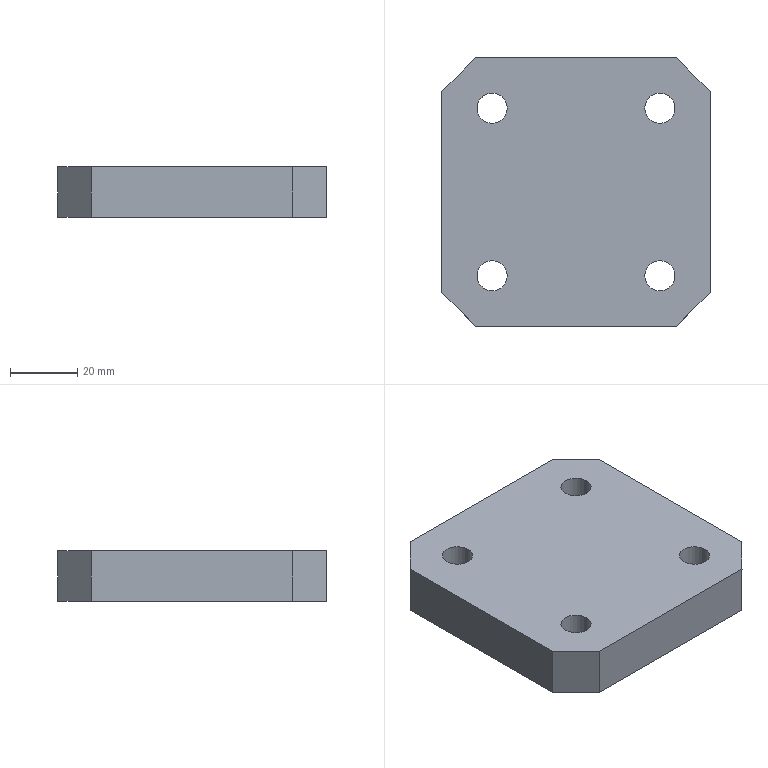Part | NX | features solid 2 | 1 solid | 14 faces | box 80 x 80 x 15 mm | volume 89183 mm3 | plane 10 | cylinder 4 | commonest cylinder face diameters 9 x4
STEP:
#1=CARTESIAN_POINT('',(-359.,-280.,315.));
#2=VERTEX_POINT('',#1);
#3=CARTESIAN_POINT('',(-419.,-280.,315.));
#4=VERTEX_POINT('',#3);
#5=CARTESIAN_POINT('',(9999577.414,-280.,315.));
#6=DIRECTION('',(-1.,0.,0.));
#7=VECTOR('',#6,1000.);
#8=LINE('',#5,#7);
#9=EDGE_CURVE('',#2,#4,#8,.T.);
#10=ORIENTED_EDGE('',*,*,#9,.T.);
#11=CARTESIAN_POINT('',(-419.,-280.,300.));
#12=VERTEX_POINT('',#11);
#13=CARTESIAN_POINT('',(-419.,-280.,300.));
#14=DIRECTION('',(0.,0.,-1.));
#15=VECTOR('',#14,1000.);
#16=LINE('',#13,#15);
#17=EDGE_CURVE('',#4,#12,#16,.T.);
#18=ORIENTED_EDGE('',*,*,#17,.T.);
#19=CARTESIAN_POINT('',(-359.,-280.,300.));
#20=VERTEX_POINT('',#19);
#21=CARTESIAN_POINT('',(9999577.414,-280.,300.));
#22=DIRECTION('',(-1.,0.,0.));
#23=VECTOR('',#22,1000.);
#24=LINE('',#21,#23);
#25=EDGE_CURVE('',#20,#12,#24,.T.);
#26=ORIENTED_EDGE('',*,*,#25,.F.);
#27=CARTESIAN_POINT('',(-359.,-280.,315.));
#28=DIRECTION('',(0.,0.,1.));
#29=VECTOR('',#28,1000.);
#30=LINE('',#27,#29);
#31=EDGE_CURVE('',#20,#2,#30,.T.);
#32=ORIENTED_EDGE('',*,*,#31,.T.);
#33=EDGE_LOOP('',(#10,#18,#26,#32));
#34=FACE_BOUND('',#33,.T.);
#35=CARTESIAN_POINT('',(9999577.414,-280.,315.));
#36=DIRECTION('',(0.,-1.,0.));
#37=DIRECTION('',(0.,0.,-1.));
#38=AXIS2_PLACEMENT_3D('',#35,#36,#37);
#39=PLANE('',#38);
#40=ADVANCED_FACE('',(#34),#39,.T.);
#41=CARTESIAN_POINT('',(-429.,-210.,300.));
#42=VERTEX_POINT('',#41);
#43=CARTESIAN_POINT('',(-429.,-270.,300.));
#44=VERTEX_POINT('',#43);
#45=CARTESIAN_POINT('',(-429.,-205.,300.));
#46=DIRECTION('',(0.,-1.,0.));
#47=VECTOR('',#46,1000.);
#48=LINE('',#45,#47);
#49=EDGE_CURVE('',#42,#44,#48,.T.);
#50=ORIENTED_EDGE('',*,*,#49,.T.);
#51=CARTESIAN_POINT('',(-429.,-270.,315.));
#52=VERTEX_POINT('',#51);
#53=CARTESIAN_POINT('',(-429.,-270.,315.));
#54=DIRECTION('',(0.,0.,1.));
#55=VECTOR('',#54,1000.);
#56=LINE('',#53,#55);
#57=EDGE_CURVE('',#44,#52,#56,.T.);
#58=ORIENTED_EDGE('',*,*,#57,.T.);
#59=CARTESIAN_POINT('',(-429.,-210.,315.));
#60=VERTEX_POINT('',#59);
#61=CARTESIAN_POINT('',(-429.,-205.,315.));
#62=DIRECTION('',(0.,-1.,0.));
#63=VECTOR('',#62,1000.);
#64=LINE('',#61,#63);
#65=EDGE_CURVE('',#60,#52,#64,.T.);
#66=ORIENTED_EDGE('',*,*,#65,.F.);
#67=CARTESIAN_POINT('',(-429.,-210.,315.));
#68=DIRECTION('',(0.,0.,-1.));
#69=VECTOR('',#68,1000.);
#70=LINE('',#67,#69);
#71=EDGE_CURVE('',#60,#42,#70,.T.);
#72=ORIENTED_EDGE('',*,*,#71,.T.);
#73=EDGE_LOOP('',(#50,#58,#66,#72));
#74=FACE_BOUND('',#73,.T.);
#75=CARTESIAN_POINT('',(-429.,-205.,315.));
#76=DIRECTION('',(1.,0.,0.));
#77=DIRECTION('',(0.,0.,-1.));
#78=AXIS2_PLACEMENT_3D('',#75,#76,#77);
#79=PLANE('',#78);
#80=ADVANCED_FACE('',(#74),#79,.F.);
#81=CARTESIAN_POINT('',(-359.,-200.,315.));
#82=VERTEX_POINT('',#81);
#83=CARTESIAN_POINT('',(-419.,-200.,315.));
#84=VERTEX_POINT('',#83);
#85=CARTESIAN_POINT('',(-359.,-200.,315.));
#86=CARTESIAN_POINT('',(-379.,-200.,315.));
#87=CARTESIAN_POINT('',(-399.,-200.,315.));
#88=CARTESIAN_POINT('',(-419.,-200.,315.));
#89=B_SPLINE_CURVE_WITH_KNOTS('',3,(#85,#86,#87,#88),.UNSPECIFIED.,.F.,.F.,(4,4),(0.125,0.875),.UNSPECIFIED.);
#90=EDGE_CURVE('',#82,#84,#89,.T.);
#91=ORIENTED_EDGE('',*,*,#90,.F.);
#92=CARTESIAN_POINT('',(-359.,-200.,300.));
#93=VERTEX_POINT('',#92);
#94=CARTESIAN_POINT('',(-359.,-200.,300.));
#95=DIRECTION('',(0.,0.,-1.));
#96=VECTOR('',#95,1000.);
#97=LINE('',#94,#96);
#98=EDGE_CURVE('',#82,#93,#97,.T.);
#99=ORIENTED_EDGE('',*,*,#98,.T.);
#100=CARTESIAN_POINT('',(-419.,-200.,300.));
#101=VERTEX_POINT('',#100);
#102=CARTESIAN_POINT('',(-419.,-200.,300.));
#103=CARTESIAN_POINT('',(-399.,-200.,300.));
#104=CARTESIAN_POINT('',(-379.,-200.,300.));
#105=CARTESIAN_POINT('',(-359.,-200.,300.));
#106=B_SPLINE_CURVE_WITH_KNOTS('',3,(#102,#103,#104,#105),.UNSPECIFIED.,.F.,.F.,(4,4),(0.125,0.875),.UNSPECIFIED.);
#107=EDGE_CURVE('',#93,#101,#106,.F.);
#108=ORIENTED_EDGE('',*,*,#107,.T.);
#109=CARTESIAN_POINT('',(-419.,-200.,315.));
#110=DIRECTION('',(0.,0.,1.));
#111=VECTOR('',#110,1000.);
#112=LINE('',#109,#111);
#113=EDGE_CURVE('',#101,#84,#112,.T.);
#114=ORIENTED_EDGE('',*,*,#113,.T.);
#115=EDGE_LOOP('',(#91,#99,#108,#114));
#116=FACE_BOUND('',#115,.T.);
#117=CARTESIAN_POINT('',(-355.414,-200.,315.));
#118=DIRECTION('',(0.,-1.,0.));
#119=DIRECTION('',(0.,0.,-1.));
#120=AXIS2_PLACEMENT_3D('',#117,#118,#119);
#121=PLANE('',#120);
#122=ADVANCED_FACE('',(#116),#121,.F.);
#123=CARTESIAN_POINT('',(-349.,-210.,315.));
#124=VERTEX_POINT('',#123);
#125=CARTESIAN_POINT('',(-349.,-270.,315.));
#126=VERTEX_POINT('',#125);
#127=CARTESIAN_POINT('',(-349.,9999726.414,315.));
#128=DIRECTION('',(0.,-1.,0.));
#129=VECTOR('',#128,1000.);
#130=LINE('',#127,#129);
#131=EDGE_CURVE('',#124,#126,#130,.T.);
#132=ORIENTED_EDGE('',*,*,#131,.T.);
#133=CARTESIAN_POINT('',(-349.,-270.,300.));
#134=VERTEX_POINT('',#133);
#135=CARTESIAN_POINT('',(-349.,-270.,315.));
#136=DIRECTION('',(0.,0.,-1.));
#137=VECTOR('',#136,1000.);
#138=LINE('',#135,#137);
#139=EDGE_CURVE('',#126,#134,#138,.T.);
#140=ORIENTED_EDGE('',*,*,#139,.T.);
#141=CARTESIAN_POINT('',(-349.,-210.,300.));
#142=VERTEX_POINT('',#141);
#143=CARTESIAN_POINT('',(-349.,9999726.414,300.));
#144=DIRECTION('',(0.,-1.,0.));
#145=VECTOR('',#144,1000.);
#146=LINE('',#143,#145);
#147=EDGE_CURVE('',#142,#134,#146,.T.);
#148=ORIENTED_EDGE('',*,*,#147,.F.);
#149=CARTESIAN_POINT('',(-349.,-210.,315.));
#150=DIRECTION('',(0.,0.,1.));
#151=VECTOR('',#150,1000.);
#152=LINE('',#149,#151);
#153=EDGE_CURVE('',#142,#124,#152,.T.);
#154=ORIENTED_EDGE('',*,*,#153,.T.);
#155=EDGE_LOOP('',(#132,#140,#148,#154));
#156=FACE_BOUND('',#155,.T.);
#157=CARTESIAN_POINT('',(-349.,9999726.414,315.));
#158=DIRECTION('',(1.,0.,0.));
#159=DIRECTION('',(0.,0.,-1.));
#160=AXIS2_PLACEMENT_3D('',#157,#158,#159);
#161=PLANE('',#160);
#162=ADVANCED_FACE('',(#156),#161,.T.);
#163=CARTESIAN_POINT('',(-359.504,-215.004,315.));
#164=VERTEX_POINT('',#163);
#165=CARTESIAN_POINT('',(-364.004,-215.004,315.));
#166=DIRECTION('',(0.,0.,1.));
#167=DIRECTION('',(1.,0.,0.));
#168=AXIS2_PLACEMENT_3D('',#165,#166,#167);
#169=CIRCLE('',#168,4.5);
#170=EDGE_CURVE('',#164,#164,#169,.T.);
#171=ORIENTED_EDGE('',*,*,#170,.F.);
#172=EDGE_LOOP('',(#171));
#173=FACE_BOUND('',#172,.T.);
#174=CARTESIAN_POINT('',(-409.496,-215.004,315.));
#175=VERTEX_POINT('',#174);
#176=CARTESIAN_POINT('',(-413.996,-215.004,315.));
#177=DIRECTION('',(0.,0.,1.));
#178=DIRECTION('',(1.,0.,0.));
#179=AXIS2_PLACEMENT_3D('',#176,#177,#178);
#180=CIRCLE('',#179,4.5);
#181=EDGE_CURVE('',#175,#175,#180,.T.);
#182=ORIENTED_EDGE('',*,*,#181,.F.);
#183=EDGE_LOOP('',(#182));
#184=FACE_BOUND('',#183,.T.);
#185=CARTESIAN_POINT('',(-409.496,-264.996,315.));
#186=VERTEX_POINT('',#185);
#187=CARTESIAN_POINT('',(-413.996,-264.996,315.));
#188=DIRECTION('',(0.,0.,1.));
#189=DIRECTION('',(1.,0.,0.));
#190=AXIS2_PLACEMENT_3D('',#187,#188,#189);
#191=CIRCLE('',#190,4.5);
#192=EDGE_CURVE('',#186,#186,#191,.T.);
#193=ORIENTED_EDGE('',*,*,#192,.F.);
#194=EDGE_LOOP('',(#193));
#195=FACE_BOUND('',#194,.T.);
#196=CARTESIAN_POINT('',(-359.504,-264.996,315.));
#197=VERTEX_POINT('',#196);
#198=CARTESIAN_POINT('',(-364.004,-264.996,315.));
#199=DIRECTION('',(0.,0.,1.));
#200=DIRECTION('',(1.,0.,0.));
#201=AXIS2_PLACEMENT_3D('',#198,#199,#200);
#202=CIRCLE('',#201,4.5);
#203=EDGE_CURVE('',#197,#197,#202,.T.);
#204=ORIENTED_EDGE('',*,*,#203,.F.);
#205=EDGE_LOOP('',(#204));
#206=FACE_BOUND('',#205,.T.);
#207=ORIENTED_EDGE('',*,*,#65,.T.);
#208=CARTESIAN_POINT('',(-424.707,-274.293,315.));
#209=DIRECTION('',(0.7071,-0.7071,0.));
#210=VECTOR('',#209,1000.);
#211=LINE('',#208,#210);
#212=EDGE_CURVE('',#52,#4,#211,.T.);
#213=ORIENTED_EDGE('',*,*,#212,.T.);
#214=ORIENTED_EDGE('',*,*,#9,.F.);
#215=CARTESIAN_POINT('',(-319.707,-240.707,315.));
#216=DIRECTION('',(-0.7071,-0.7071,0.));
#217=VECTOR('',#216,1000.);
#218=LINE('',#215,#217);
#219=EDGE_CURVE('',#2,#126,#218,.F.);
#220=ORIENTED_EDGE('',*,*,#219,.T.);
#221=ORIENTED_EDGE('',*,*,#131,.F.);
#222=CARTESIAN_POINT('',(-354.707,-204.293,315.));
#223=DIRECTION('',(-0.7071,0.7071,0.));
#224=VECTOR('',#223,1000.);
#225=LINE('',#222,#224);
#226=EDGE_CURVE('',#124,#82,#225,.T.);
#227=ORIENTED_EDGE('',*,*,#226,.T.);
#228=ORIENTED_EDGE('',*,*,#90,.T.);
#229=CARTESIAN_POINT('',(-389.707,-170.707,315.));
#230=DIRECTION('',(0.7071,0.7071,0.));
#231=VECTOR('',#230,1000.);
#232=LINE('',#229,#231);
#233=EDGE_CURVE('',#84,#60,#232,.F.);
#234=ORIENTED_EDGE('',*,*,#233,.T.);
#235=EDGE_LOOP('',(#207,#213,#214,#220,#221,#227,#228,#234));
#236=FACE_BOUND('',#235,.T.);
#237=CARTESIAN_POINT('',(-355.414,-205.,315.));
#238=DIRECTION('',(0.,0.,1.));
#239=DIRECTION('',(-1.,0.,0.));
#240=AXIS2_PLACEMENT_3D('',#237,#238,#239);
#241=PLANE('',#240);
#242=ADVANCED_FACE('',(#173,#184,#195,#206,#236),#241,.T.);
#243=CARTESIAN_POINT('',(-359.504,-215.004,300.));
#244=VERTEX_POINT('',#243);
#245=CARTESIAN_POINT('',(-364.004,-215.004,300.));
#246=DIRECTION('',(0.,0.,1.));
#247=DIRECTION('',(1.,0.,0.));
#248=AXIS2_PLACEMENT_3D('',#245,#246,#247);
#249=CIRCLE('',#248,4.5);
#250=EDGE_CURVE('',#244,#244,#249,.T.);
#251=ORIENTED_EDGE('',*,*,#250,.T.);
#252=EDGE_LOOP('',(#251));
#253=FACE_BOUND('',#252,.T.);
#254=CARTESIAN_POINT('',(-409.496,-215.004,300.));
#255=VERTEX_POINT('',#254);
#256=CARTESIAN_POINT('',(-413.996,-215.004,300.));
#257=DIRECTION('',(0.,0.,1.));
#258=DIRECTION('',(1.,0.,0.));
#259=AXIS2_PLACEMENT_3D('',#256,#257,#258);
#260=CIRCLE('',#259,4.5);
#261=EDGE_CURVE('',#255,#255,#260,.T.);
#262=ORIENTED_EDGE('',*,*,#261,.T.);
#263=EDGE_LOOP('',(#262));
#264=FACE_BOUND('',#263,.T.);
#265=CARTESIAN_POINT('',(-409.496,-264.996,300.));
#266=VERTEX_POINT('',#265);
#267=CARTESIAN_POINT('',(-413.996,-264.996,300.));
#268=DIRECTION('',(0.,0.,1.));
#269=DIRECTION('',(1.,0.,0.));
#270=AXIS2_PLACEMENT_3D('',#267,#268,#269);
#271=CIRCLE('',#270,4.5);
#272=EDGE_CURVE('',#266,#266,#271,.T.);
#273=ORIENTED_EDGE('',*,*,#272,.T.);
#274=EDGE_LOOP('',(#273));
#275=FACE_BOUND('',#274,.T.);
#276=CARTESIAN_POINT('',(-359.504,-264.996,300.));
#277=VERTEX_POINT('',#276);
#278=CARTESIAN_POINT('',(-364.004,-264.996,300.));
#279=DIRECTION('',(0.,0.,1.));
#280=DIRECTION('',(1.,0.,0.));
#281=AXIS2_PLACEMENT_3D('',#278,#279,#280);
#282=CIRCLE('',#281,4.5);
#283=EDGE_CURVE('',#277,#277,#282,.T.);
#284=ORIENTED_EDGE('',*,*,#283,.T.);
#285=EDGE_LOOP('',(#284));
#286=FACE_BOUND('',#285,.T.);
#287=ORIENTED_EDGE('',*,*,#25,.T.);
#288=CARTESIAN_POINT('',(-419.,-280.,300.));
#289=DIRECTION('',(-0.7071,0.7071,0.));
#290=VECTOR('',#289,1000.);
#291=LINE('',#288,#290);
#292=EDGE_CURVE('',#12,#44,#291,.T.);
#293=ORIENTED_EDGE('',*,*,#292,.T.);
#294=ORIENTED_EDGE('',*,*,#49,.F.);
#295=CARTESIAN_POINT('',(-429.,-210.,300.));
#296=DIRECTION('',(-0.7071,-0.7071,0.));
#297=VECTOR('',#296,1000.);
#298=LINE('',#295,#297);
#299=EDGE_CURVE('',#42,#101,#298,.F.);
#300=ORIENTED_EDGE('',*,*,#299,.T.);
#301=ORIENTED_EDGE('',*,*,#107,.F.);
#302=CARTESIAN_POINT('',(-359.,-200.,300.));
#303=DIRECTION('',(0.7071,-0.7071,0.));
#304=VECTOR('',#303,1000.);
#305=LINE('',#302,#304);
#306=EDGE_CURVE('',#93,#142,#305,.T.);
#307=ORIENTED_EDGE('',*,*,#306,.T.);
#308=ORIENTED_EDGE('',*,*,#147,.T.);
#309=CARTESIAN_POINT('',(-349.,-270.,300.));
#310=DIRECTION('',(0.7071,0.7071,0.));
#311=VECTOR('',#310,1000.);
#312=LINE('',#309,#311);
#313=EDGE_CURVE('',#134,#20,#312,.F.);
#314=ORIENTED_EDGE('',*,*,#313,.T.);
#315=EDGE_LOOP('',(#287,#293,#294,#300,#301,#307,#308,#314));
#316=FACE_BOUND('',#315,.T.);
#317=CARTESIAN_POINT('',(-355.414,-205.,300.));
#318=DIRECTION('',(0.,0.,1.));
#319=DIRECTION('',(-1.,0.,0.));
#320=AXIS2_PLACEMENT_3D('',#317,#318,#319);
#321=PLANE('',#320);
#322=ADVANCED_FACE('',(#253,#264,#275,#286,#316),#321,.F.);
#323=ORIENTED_EDGE('',*,*,#212,.F.);
#324=ORIENTED_EDGE('',*,*,#57,.F.);
#325=ORIENTED_EDGE('',*,*,#292,.F.);
#326=ORIENTED_EDGE('',*,*,#17,.F.);
#327=EDGE_LOOP('',(#323,#324,#325,#326));
#328=FACE_BOUND('',#327,.T.);
#329=CARTESIAN_POINT('',(-419.,-280.,315.));
#330=DIRECTION('',(-0.7071,-0.7071,0.));
#331=DIRECTION('',(0.7071,-0.7071,0.));
#332=AXIS2_PLACEMENT_3D('',#329,#330,#331);
#333=PLANE('',#332);
#334=ADVANCED_FACE('',(#328),#333,.T.);
#335=ORIENTED_EDGE('',*,*,#219,.F.);
#336=ORIENTED_EDGE('',*,*,#31,.F.);
#337=ORIENTED_EDGE('',*,*,#313,.F.);
#338=ORIENTED_EDGE('',*,*,#139,.F.);
#339=EDGE_LOOP('',(#335,#336,#337,#338));
#340=FACE_BOUND('',#339,.T.);
#341=CARTESIAN_POINT('',(-349.,-270.,315.));
#342=DIRECTION('',(-0.7071,0.7071,0.));
#343=DIRECTION('',(-0.7071,-0.7071,0.));
#344=AXIS2_PLACEMENT_3D('',#341,#342,#343);
#345=PLANE('',#344);
#346=ADVANCED_FACE('',(#340),#345,.F.);
#347=ORIENTED_EDGE('',*,*,#226,.F.);
#348=ORIENTED_EDGE('',*,*,#153,.F.);
#349=ORIENTED_EDGE('',*,*,#306,.F.);
#350=ORIENTED_EDGE('',*,*,#98,.F.);
#351=EDGE_LOOP('',(#347,#348,#349,#350));
#352=FACE_BOUND('',#351,.T.);
#353=CARTESIAN_POINT('',(-359.,-200.,315.));
#354=DIRECTION('',(0.7071,0.7071,0.));
#355=DIRECTION('',(-0.7071,0.7071,0.));
#356=AXIS2_PLACEMENT_3D('',#353,#354,#355);
#357=PLANE('',#356);
#358=ADVANCED_FACE('',(#352),#357,.T.);
#359=ORIENTED_EDGE('',*,*,#233,.F.);
#360=ORIENTED_EDGE('',*,*,#113,.F.);
#361=ORIENTED_EDGE('',*,*,#299,.F.);
#362=ORIENTED_EDGE('',*,*,#71,.F.);
#363=EDGE_LOOP('',(#359,#360,#361,#362));
#364=FACE_BOUND('',#363,.T.);
#365=CARTESIAN_POINT('',(-429.,-210.,315.));
#366=DIRECTION('',(0.7071,-0.7071,0.));
#367=DIRECTION('',(0.7071,0.7071,0.));
#368=AXIS2_PLACEMENT_3D('',#365,#366,#367);
#369=PLANE('',#368);
#370=ADVANCED_FACE('',(#364),#369,.F.);
#371=ORIENTED_EDGE('',*,*,#203,.T.);
#372=EDGE_LOOP('',(#371));
#373=FACE_BOUND('',#372,.T.);
#374=ORIENTED_EDGE('',*,*,#283,.F.);
#375=EDGE_LOOP('',(#374));
#376=FACE_BOUND('',#375,.T.);
#377=CARTESIAN_POINT('',(-364.004,-264.996,93.5));
#378=DIRECTION('',(0.,0.,1.));
#379=DIRECTION('',(1.,0.,0.));
#380=AXIS2_PLACEMENT_3D('',#377,#378,#379);
#381=CYLINDRICAL_SURFACE('',#380,4.5);
#382=ADVANCED_FACE('',(#373,#376),#381,.F.);
#383=ORIENTED_EDGE('',*,*,#192,.T.);
#384=EDGE_LOOP('',(#383));
#385=FACE_BOUND('',#384,.T.);
#386=ORIENTED_EDGE('',*,*,#272,.F.);
#387=EDGE_LOOP('',(#386));
#388=FACE_BOUND('',#387,.T.);
#389=CARTESIAN_POINT('',(-413.996,-264.996,93.5));
#390=DIRECTION('',(0.,0.,1.));
#391=DIRECTION('',(1.,0.,0.));
#392=AXIS2_PLACEMENT_3D('',#389,#390,#391);
#393=CYLINDRICAL_SURFACE('',#392,4.5);
#394=ADVANCED_FACE('',(#385,#388),#393,.F.);
#395=ORIENTED_EDGE('',*,*,#181,.T.);
#396=EDGE_LOOP('',(#395));
#397=FACE_BOUND('',#396,.T.);
#398=ORIENTED_EDGE('',*,*,#261,.F.);
#399=EDGE_LOOP('',(#398));
#400=FACE_BOUND('',#399,.T.);
#401=CARTESIAN_POINT('',(-413.996,-215.004,93.5));
#402=DIRECTION('',(0.,0.,1.));
#403=DIRECTION('',(1.,0.,0.));
#404=AXIS2_PLACEMENT_3D('',#401,#402,#403);
#405=CYLINDRICAL_SURFACE('',#404,4.5);
#406=ADVANCED_FACE('',(#397,#400),#405,.F.);
#407=ORIENTED_EDGE('',*,*,#170,.T.);
#408=EDGE_LOOP('',(#407));
#409=FACE_BOUND('',#408,.T.);
#410=ORIENTED_EDGE('',*,*,#250,.F.);
#411=EDGE_LOOP('',(#410));
#412=FACE_BOUND('',#411,.T.);
#413=CARTESIAN_POINT('',(-364.004,-215.004,93.5));
#414=DIRECTION('',(0.,0.,1.));
#415=DIRECTION('',(1.,0.,0.));
#416=AXIS2_PLACEMENT_3D('',#413,#414,#415);
#417=CYLINDRICAL_SURFACE('',#416,4.5);
#418=ADVANCED_FACE('',(#409,#412),#417,.F.);
#419=CLOSED_SHELL('',(#40,#80,#122,#162,#242,#322,#334,#346,#358,#370,#382,#394,#406,#418));
#420=MANIFOLD_SOLID_BREP('',#419);
#421=(LENGTH_UNIT()NAMED_UNIT(*)SI_UNIT(.MILLI.,.METRE.));
#422=UNCERTAINTY_MEASURE_WITH_UNIT(LENGTH_MEASURE(0.0508),#421,'','');
#423=(NAMED_UNIT(*)PLANE_ANGLE_UNIT()SI_UNIT($,.RADIAN.));
#424=(NAMED_UNIT(*)SI_UNIT($,.STERADIAN.)SOLID_ANGLE_UNIT());
#425=(GEOMETRIC_REPRESENTATION_CONTEXT(3)GLOBAL_UNCERTAINTY_ASSIGNED_CONTEXT((#422))GLOBAL_UNIT_ASSIGNED_CONTEXT((#421,#423,#424))REPRESENTATION_CONTEXT('',''));
#426=ADVANCED_BREP_SHAPE_REPRESENTATION('',(#420),#425);